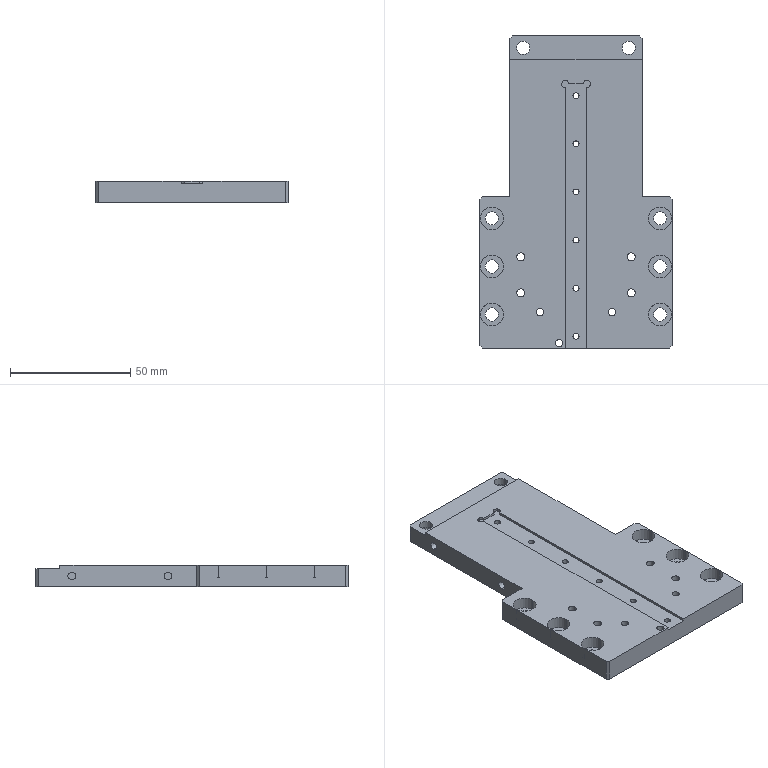Part | STEP file | PN_0069 Mount electronic clip s longitudinal manipulator base plate | 1 solid | 103 faces | box 80 x 130 x 9 mm | volume 72069 mm3 | cylinder 69 | plane 34 | commonest cylinder face diameters 3.3 x16 5.5 x16 9.5 x16 2.5 x12 3 x9